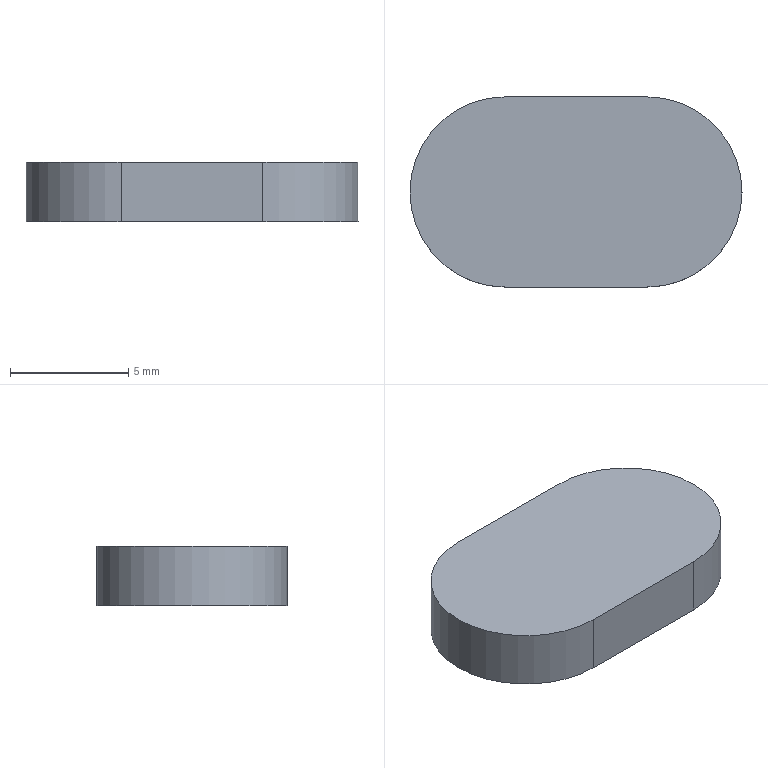Part | STEP file | lll_id1302_x_t | 1 solid | 6 faces | box 14.05 x 8.05 x 2.5 mm | volume 247.989 mm3 | plane 4 | cylinder 2 | commonest cylinder face diameters 8.05 x2
STEP:
#1=CARTESIAN_POINT('',(3584.234,234.475,0.00001673));
#2=VERTEX_POINT('',#1);
#3=CARTESIAN_POINT('',(3584.234,226.425,0.00001673));
#4=VERTEX_POINT('',#3);
#5=CARTESIAN_POINT('',(3584.234,230.45,0.00001673));
#6=DIRECTION('',(-0.000000008,0.,1.));
#7=DIRECTION('',(1.,0.,0.000000008));
#8=AXIS2_PLACEMENT_3D('',#5,#6,#7);
#9=CIRCLE('',#8,4.025);
#10=EDGE_CURVE('',#2,#4,#9,.T.);
#11=ORIENTED_EDGE('',*,*,#10,.T.);
#12=CARTESIAN_POINT('',(3584.234,226.425,2.5));
#13=VERTEX_POINT('',#12);
#14=CARTESIAN_POINT('',(3584.234,226.425,2.5));
#15=DIRECTION('',(0.000000008,0.,-1.));
#16=VECTOR('',#15,1.);
#17=LINE('',#14,#16);
#18=EDGE_CURVE('',#13,#4,#17,.T.);
#19=ORIENTED_EDGE('',*,*,#18,.F.);
#20=CARTESIAN_POINT('',(3584.234,234.475,2.5));
#21=VERTEX_POINT('',#20);
#22=CARTESIAN_POINT('',(3584.234,230.45,2.5));
#23=DIRECTION('',(-0.000000008,0.,1.));
#24=DIRECTION('',(-1.,0.,-0.000000008));
#25=AXIS2_PLACEMENT_3D('',#22,#23,#24);
#26=CIRCLE('',#25,4.025);
#27=EDGE_CURVE('',#21,#13,#26,.T.);
#28=ORIENTED_EDGE('',*,*,#27,.F.);
#29=CARTESIAN_POINT('',(3584.234,234.475,2.5));
#30=DIRECTION('',(-0.000000008,0.,1.));
#31=VECTOR('',#30,1.);
#32=LINE('',#29,#31);
#33=EDGE_CURVE('',#2,#21,#32,.T.);
#34=ORIENTED_EDGE('',*,*,#33,.F.);
#35=EDGE_LOOP('',(#11,#19,#28,#34));
#36=FACE_OUTER_BOUND('',#35,.T.);
#37=CARTESIAN_POINT('',(3584.234,230.45,2.5));
#38=DIRECTION('',(0.000000008,0.,-1.));
#39=DIRECTION('',(0.,1.,0.));
#40=AXIS2_PLACEMENT_3D('',#37,#38,#39);
#41=CYLINDRICAL_SURFACE('',#40,4.025);
#42=ADVANCED_FACE('',(#36),#41,.T.);
#43=ORIENTED_EDGE('',*,*,#27,.T.);
#44=CARTESIAN_POINT('',(3590.234,226.425,2.5));
#45=VERTEX_POINT('',#44);
#46=CARTESIAN_POINT('',(3584.234,226.425,2.5));
#47=DIRECTION('',(1.,0.,0.000000008));
#48=VECTOR('',#47,1.);
#49=LINE('',#46,#48);
#50=EDGE_CURVE('',#13,#45,#49,.T.);
#51=ORIENTED_EDGE('',*,*,#50,.T.);
#52=CARTESIAN_POINT('',(3590.234,234.475,2.5));
#53=VERTEX_POINT('',#52);
#54=CARTESIAN_POINT('',(3590.234,230.45,2.5));
#55=DIRECTION('',(-0.000000008,0.,1.));
#56=DIRECTION('',(-1.,0.,-0.000000008));
#57=AXIS2_PLACEMENT_3D('',#54,#55,#56);
#58=CIRCLE('',#57,4.025);
#59=EDGE_CURVE('',#45,#53,#58,.T.);
#60=ORIENTED_EDGE('',*,*,#59,.T.);
#61=CARTESIAN_POINT('',(3584.234,234.475,2.5));
#62=DIRECTION('',(1.,0.,0.000000008));
#63=VECTOR('',#62,1.);
#64=LINE('',#61,#63);
#65=EDGE_CURVE('',#21,#53,#64,.T.);
#66=ORIENTED_EDGE('',*,*,#65,.F.);
#67=EDGE_LOOP('',(#43,#51,#60,#66));
#68=FACE_OUTER_BOUND('',#67,.T.);
#69=CARTESIAN_POINT('',(3584.234,230.45,2.5));
#70=DIRECTION('',(-0.000000008,0.,1.));
#71=DIRECTION('',(0.,-1.,0.));
#72=AXIS2_PLACEMENT_3D('',#69,#70,#71);
#73=PLANE('',#72);
#74=ADVANCED_FACE('',(#68),#73,.T.);
#75=ORIENTED_EDGE('',*,*,#10,.F.);
#76=CARTESIAN_POINT('',(3590.234,234.475,0.00001673));
#77=VERTEX_POINT('',#76);
#78=CARTESIAN_POINT('',(3584.234,234.475,0.00001673));
#79=DIRECTION('',(1.,0.,0.000000008));
#80=VECTOR('',#79,1.);
#81=LINE('',#78,#80);
#82=EDGE_CURVE('',#2,#77,#81,.T.);
#83=ORIENTED_EDGE('',*,*,#82,.T.);
#84=CARTESIAN_POINT('',(3590.234,226.425,0.00001673));
#85=VERTEX_POINT('',#84);
#86=CARTESIAN_POINT('',(3590.234,230.45,0.00001678));
#87=DIRECTION('',(-0.000000008,0.,1.));
#88=DIRECTION('',(1.,0.,0.000000008));
#89=AXIS2_PLACEMENT_3D('',#86,#87,#88);
#90=CIRCLE('',#89,4.025);
#91=EDGE_CURVE('',#85,#77,#90,.T.);
#92=ORIENTED_EDGE('',*,*,#91,.F.);
#93=CARTESIAN_POINT('',(3584.234,226.425,0.00001673));
#94=DIRECTION('',(1.,0.,0.000000008));
#95=VECTOR('',#94,1.);
#96=LINE('',#93,#95);
#97=EDGE_CURVE('',#4,#85,#96,.T.);
#98=ORIENTED_EDGE('',*,*,#97,.F.);
#99=EDGE_LOOP('',(#75,#83,#92,#98));
#100=FACE_OUTER_BOUND('',#99,.T.);
#101=CARTESIAN_POINT('',(3584.234,230.45,0.00001673));
#102=DIRECTION('',(0.000000008,0.,-1.));
#103=DIRECTION('',(0.,1.,0.));
#104=AXIS2_PLACEMENT_3D('',#101,#102,#103);
#105=PLANE('',#104);
#106=ADVANCED_FACE('',(#100),#105,.T.);
#107=CARTESIAN_POINT('',(3590.234,226.425,2.5));
#108=DIRECTION('',(-0.000000008,0.,1.));
#109=VECTOR('',#108,1.);
#110=LINE('',#107,#109);
#111=EDGE_CURVE('',#85,#45,#110,.T.);
#112=ORIENTED_EDGE('',*,*,#111,.F.);
#113=ORIENTED_EDGE('',*,*,#91,.T.);
#114=CARTESIAN_POINT('',(3590.234,234.475,2.5));
#115=DIRECTION('',(0.000000008,0.,-1.));
#116=VECTOR('',#115,1.);
#117=LINE('',#114,#116);
#118=EDGE_CURVE('',#53,#77,#117,.T.);
#119=ORIENTED_EDGE('',*,*,#118,.F.);
#120=ORIENTED_EDGE('',*,*,#59,.F.);
#121=EDGE_LOOP('',(#112,#113,#119,#120));
#122=FACE_OUTER_BOUND('',#121,.T.);
#123=CARTESIAN_POINT('',(3590.234,230.45,2.5));
#124=DIRECTION('',(0.000000008,0.,-1.));
#125=DIRECTION('',(0.,1.,0.));
#126=AXIS2_PLACEMENT_3D('',#123,#124,#125);
#127=CYLINDRICAL_SURFACE('',#126,4.025);
#128=ADVANCED_FACE('',(#122),#127,.T.);
#129=ORIENTED_EDGE('',*,*,#118,.T.);
#130=ORIENTED_EDGE('',*,*,#82,.F.);
#131=ORIENTED_EDGE('',*,*,#33,.T.);
#132=ORIENTED_EDGE('',*,*,#65,.T.);
#133=EDGE_LOOP('',(#129,#130,#131,#132));
#134=FACE_OUTER_BOUND('',#133,.T.);
#135=CARTESIAN_POINT('',(3584.234,234.475,2.5));
#136=DIRECTION('',(0.,-1.,0.));
#137=DIRECTION('',(0.,0.,1.));
#138=AXIS2_PLACEMENT_3D('',#135,#136,#137);
#139=PLANE('',#138);
#140=ADVANCED_FACE('',(#134),#139,.F.);
#141=ORIENTED_EDGE('',*,*,#111,.T.);
#142=ORIENTED_EDGE('',*,*,#50,.F.);
#143=ORIENTED_EDGE('',*,*,#18,.T.);
#144=ORIENTED_EDGE('',*,*,#97,.T.);
#145=EDGE_LOOP('',(#141,#142,#143,#144));
#146=FACE_OUTER_BOUND('',#145,.T.);
#147=CARTESIAN_POINT('',(3584.234,226.425,0.00001669));
#148=DIRECTION('',(0.,1.,0.));
#149=DIRECTION('',(0.,0.,-1.));
#150=AXIS2_PLACEMENT_3D('',#147,#148,#149);
#151=PLANE('',#150);
#152=ADVANCED_FACE('',(#146),#151,.F.);
#153=CLOSED_SHELL('',(#42,#74,#106,#128,#140,#152));
#154=MANIFOLD_SOLID_BREP('',#153);
#155=(LENGTH_UNIT()NAMED_UNIT(*)SI_UNIT(.MILLI.,.METRE.));
#156=UNCERTAINTY_MEASURE_WITH_UNIT(LENGTH_MEASURE(0.00002),#155,'','');
#157=(NAMED_UNIT(*)PLANE_ANGLE_UNIT()SI_UNIT($,.RADIAN.));
#158=PLANE_ANGLE_MEASURE_WITH_UNIT(PLANE_ANGLE_MEASURE(0.01745),#157);
#159=DIMENSIONAL_EXPONENTS(0.,0.,0.,0.,0.,0.,0.);
#160=(CONVERSION_BASED_UNIT('DEGREE',#158)NAMED_UNIT(#159)PLANE_ANGLE_UNIT());
#161=(NAMED_UNIT(*)SI_UNIT($,.STERADIAN.)SOLID_ANGLE_UNIT());
#162=(GEOMETRIC_REPRESENTATION_CONTEXT(3)GLOBAL_UNCERTAINTY_ASSIGNED_CONTEXT((#156))GLOBAL_UNIT_ASSIGNED_CONTEXT((#155,#160,#161))REPRESENTATION_CONTEXT('',''));
#163=ADVANCED_BREP_SHAPE_REPRESENTATION('',(#154),#162);